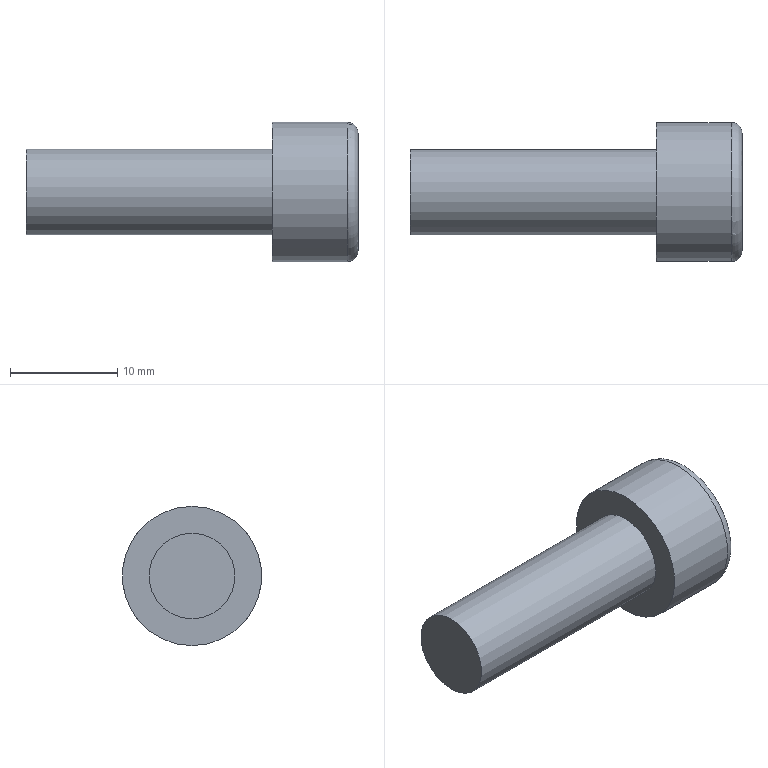Part | STEP file | Tube feed_id542_x_t | 1 solid | 19 faces | box 31 x 13 x 13 mm | volume 2040 mm3 | plane 10 | cylinder 8 | torus 1 | commonest cylinder face diameters 2 x6 8 x1 13 x1